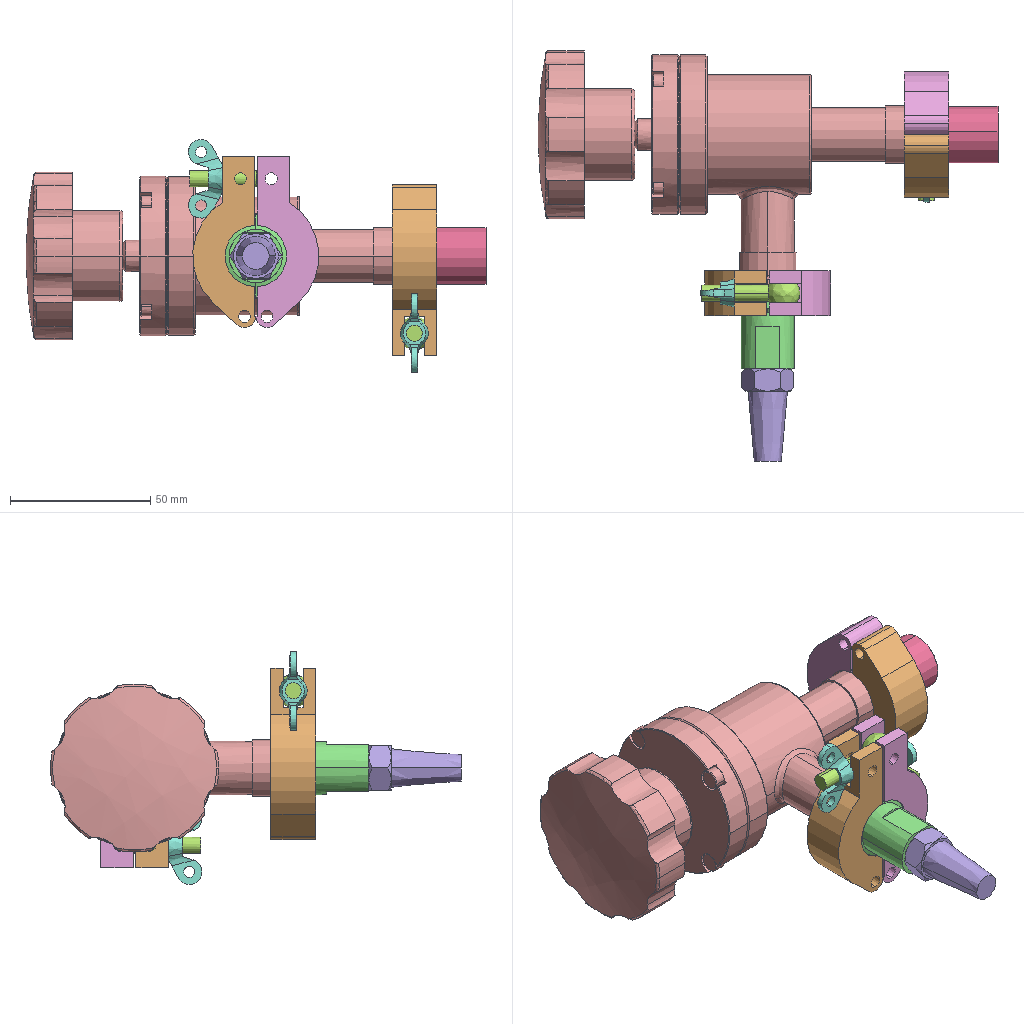Assembly | SolidWorks | 6 different items | 8 placed | box 164 x 146 x 83 mm
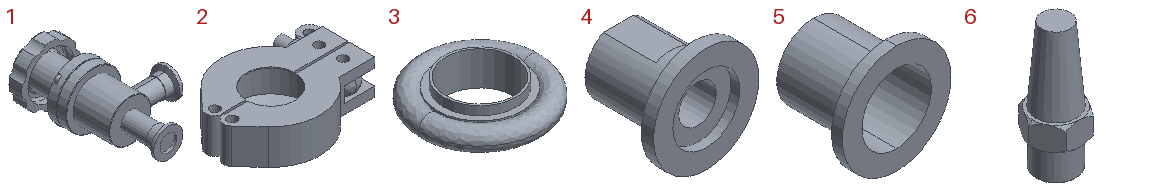Parts list (item | quantity | size | volume | features):
1 | x1 | 84.6 x 136.5 x 60.001 mm | 174648 mm3 | features BaseBody 1
2 | x2 | 67 x 46.5 x 16 mm | 18231 mm3 | features BaseBody 4
3 | x2 | 29 x 29 x 8 mm | 1965 mm3 | features BaseBody 1
4 | x1 | 30 x 25 x 30 mm | 5740 mm3 | features BaseBody 1
5 | x1 | 30 x 23 x 30 mm | 1871 mm3 | features ICE 2, Extrusion 1
6 | x1 | 18.475 x 16 x 43 mm | 4994 mm3 | features BaseBody 1
Mates (type | each side: item.copy, entity, surface, feature):
Concentric | 3.1 edge | 5.1 edge
Tangent | 3.1 face surface:4010 Input 1 | 5.1 face plane Boss-Extrude2